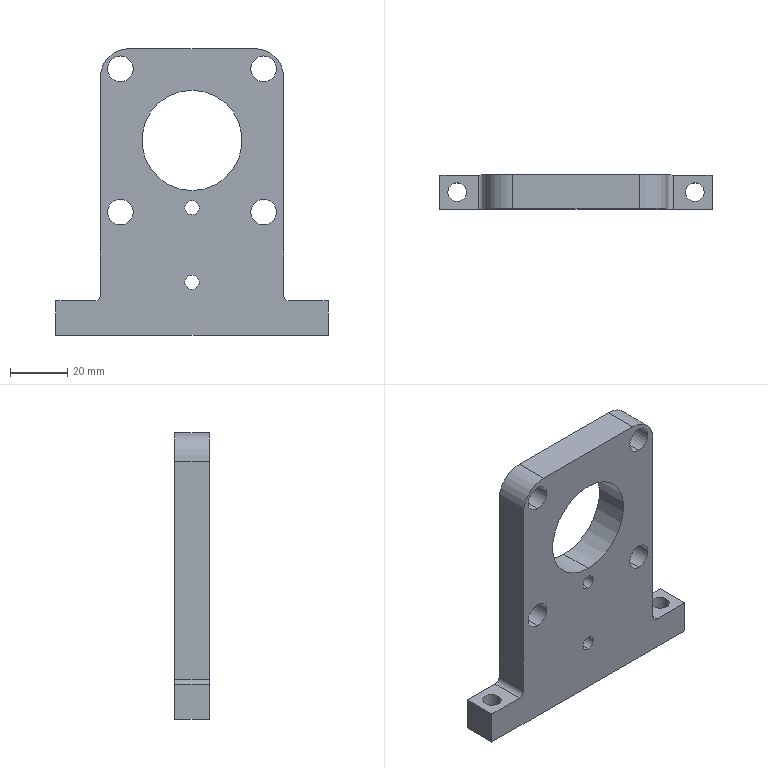Part | SolidWorks | features HoleWzd 6, ICE 3, Fillet 2, Extrusion 1 | 1 solid | 40 faces | box 95 x 12 x 100 mm | volume 64491 mm3 | cylinder 26 | plane 10 | cone 4 | commonest cylinder face diameters 5 x8 9 x8 6.5 x4 4 x2 20 x2 35 x2
STEP:
#1=CARTESIAN_POINT('',(47.5,12.,21.));
#2=VERTEX_POINT('',#1);
#3=CARTESIAN_POINT('',(47.5,12.,16.));
#4=VERTEX_POINT('',#3);
#5=CARTESIAN_POINT('',(47.5,12.,18.5));
#6=DIRECTION('',(0.,-1.,0.));
#7=DIRECTION('',(0.,0.,-1.));
#8=AXIS2_PLACEMENT_3D('',#5,#6,#7);
#9=CIRCLE('',#8,2.5);
#10=EDGE_CURVE('',#2,#4,#9,.T.);
#11=ORIENTED_EDGE('',*,*,#10,.F.);
#12=CARTESIAN_POINT('',(47.5,0.,21.));
#13=VERTEX_POINT('',#12);
#14=CARTESIAN_POINT('',(47.5,0.,21.));
#15=DIRECTION('',(0.,-1.,0.));
#16=VECTOR('',#15,1000.);
#17=LINE('',#14,#16);
#18=EDGE_CURVE('',#2,#13,#17,.T.);
#19=ORIENTED_EDGE('',*,*,#18,.T.);
#20=CARTESIAN_POINT('',(47.5,0.,16.));
#21=VERTEX_POINT('',#20);
#22=CARTESIAN_POINT('',(47.5,0.,18.5));
#23=DIRECTION('',(0.,-1.,0.));
#24=DIRECTION('',(0.,0.,-1.));
#25=AXIS2_PLACEMENT_3D('',#22,#23,#24);
#26=CIRCLE('',#25,2.5);
#27=EDGE_CURVE('',#13,#21,#26,.T.);
#28=ORIENTED_EDGE('',*,*,#27,.T.);
#29=CARTESIAN_POINT('',(47.5,0.,16.));
#30=DIRECTION('',(0.,-1.,0.));
#31=VECTOR('',#30,1000.);
#32=LINE('',#29,#31);
#33=EDGE_CURVE('',#4,#21,#32,.T.);
#34=ORIENTED_EDGE('',*,*,#33,.F.);
#35=EDGE_LOOP('',(#11,#19,#28,#34));
#36=FACE_OUTER_BOUND('',#35,.T.);
#37=CARTESIAN_POINT('',(47.5,0.,18.5));
#38=DIRECTION('',(0.,-1.,0.));
#39=DIRECTION('',(0.,0.,-1.));
#40=AXIS2_PLACEMENT_3D('',#37,#38,#39);
#41=CYLINDRICAL_SURFACE('',#40,2.5);
#42=ADVANCED_FACE('',(#36),#41,.F.);
#43=CARTESIAN_POINT('',(47.5,12.,47.));
#44=VERTEX_POINT('',#43);
#45=CARTESIAN_POINT('',(47.5,12.,42.));
#46=VERTEX_POINT('',#45);
#47=CARTESIAN_POINT('',(47.5,12.,44.5));
#48=DIRECTION('',(0.,-1.,0.));
#49=DIRECTION('',(0.,0.,-1.));
#50=AXIS2_PLACEMENT_3D('',#47,#48,#49);
#51=CIRCLE('',#50,2.5);
#52=EDGE_CURVE('',#44,#46,#51,.T.);
#53=ORIENTED_EDGE('',*,*,#52,.F.);
#54=CARTESIAN_POINT('',(47.5,0.,47.));
#55=VERTEX_POINT('',#54);
#56=CARTESIAN_POINT('',(47.5,0.,47.));
#57=DIRECTION('',(0.,-1.,0.));
#58=VECTOR('',#57,1000.);
#59=LINE('',#56,#58);
#60=EDGE_CURVE('',#44,#55,#59,.T.);
#61=ORIENTED_EDGE('',*,*,#60,.T.);
#62=CARTESIAN_POINT('',(47.5,0.,42.));
#63=VERTEX_POINT('',#62);
#64=CARTESIAN_POINT('',(47.5,0.,44.5));
#65=DIRECTION('',(0.,-1.,0.));
#66=DIRECTION('',(0.,0.,-1.));
#67=AXIS2_PLACEMENT_3D('',#64,#65,#66);
#68=CIRCLE('',#67,2.5);
#69=EDGE_CURVE('',#55,#63,#68,.T.);
#70=ORIENTED_EDGE('',*,*,#69,.T.);
#71=CARTESIAN_POINT('',(47.5,0.,42.));
#72=DIRECTION('',(0.,-1.,0.));
#73=VECTOR('',#72,1000.);
#74=LINE('',#71,#73);
#75=EDGE_CURVE('',#46,#63,#74,.T.);
#76=ORIENTED_EDGE('',*,*,#75,.F.);
#77=EDGE_LOOP('',(#53,#61,#70,#76));
#78=FACE_OUTER_BOUND('',#77,.T.);
#79=CARTESIAN_POINT('',(47.5,0.,44.5));
#80=DIRECTION('',(0.,-1.,0.));
#81=DIRECTION('',(0.,0.,-1.));
#82=AXIS2_PLACEMENT_3D('',#79,#80,#81);
#83=CYLINDRICAL_SURFACE('',#82,2.5);
#84=ADVANCED_FACE('',(#78),#83,.F.);
#85=CARTESIAN_POINT('',(72.5,12.,47.5));
#86=VERTEX_POINT('',#85);
#87=CARTESIAN_POINT('',(72.5,12.,38.5));
#88=VERTEX_POINT('',#87);
#89=CARTESIAN_POINT('',(72.5,12.,43.));
#90=DIRECTION('',(0.,-1.,0.));
#91=DIRECTION('',(0.,0.,-1.));
#92=AXIS2_PLACEMENT_3D('',#89,#90,#91);
#93=CIRCLE('',#92,4.5);
#94=EDGE_CURVE('',#86,#88,#93,.T.);
#95=ORIENTED_EDGE('',*,*,#94,.F.);
#96=CARTESIAN_POINT('',(72.5,0.,47.5));
#97=VERTEX_POINT('',#96);
#98=CARTESIAN_POINT('',(72.5,0.,47.5));
#99=DIRECTION('',(0.,-1.,0.));
#100=VECTOR('',#99,1000.);
#101=LINE('',#98,#100);
#102=EDGE_CURVE('',#86,#97,#101,.T.);
#103=ORIENTED_EDGE('',*,*,#102,.T.);
#104=CARTESIAN_POINT('',(72.5,0.,38.5));
#105=VERTEX_POINT('',#104);
#106=CARTESIAN_POINT('',(72.5,0.,43.));
#107=DIRECTION('',(0.,-1.,0.));
#108=DIRECTION('',(0.,0.,-1.));
#109=AXIS2_PLACEMENT_3D('',#106,#107,#108);
#110=CIRCLE('',#109,4.5);
#111=EDGE_CURVE('',#97,#105,#110,.T.);
#112=ORIENTED_EDGE('',*,*,#111,.T.);
#113=CARTESIAN_POINT('',(72.5,0.,38.5));
#114=DIRECTION('',(0.,-1.,0.));
#115=VECTOR('',#114,1000.);
#116=LINE('',#113,#115);
#117=EDGE_CURVE('',#88,#105,#116,.T.);
#118=ORIENTED_EDGE('',*,*,#117,.F.);
#119=EDGE_LOOP('',(#95,#103,#112,#118));
#120=FACE_OUTER_BOUND('',#119,.T.);
#121=CARTESIAN_POINT('',(72.5,0.,43.));
#122=DIRECTION('',(0.,-1.,0.));
#123=DIRECTION('',(0.,0.,-1.));
#124=AXIS2_PLACEMENT_3D('',#121,#122,#123);
#125=CYLINDRICAL_SURFACE('',#124,4.5);
#126=ADVANCED_FACE('',(#120),#125,.F.);
#127=CARTESIAN_POINT('',(72.5,12.,97.5));
#128=VERTEX_POINT('',#127);
#129=CARTESIAN_POINT('',(72.5,12.,88.5));
#130=VERTEX_POINT('',#129);
#131=CARTESIAN_POINT('',(72.5,12.,93.));
#132=DIRECTION('',(0.,-1.,0.));
#133=DIRECTION('',(0.,0.,-1.));
#134=AXIS2_PLACEMENT_3D('',#131,#132,#133);
#135=CIRCLE('',#134,4.5);
#136=EDGE_CURVE('',#128,#130,#135,.T.);
#137=ORIENTED_EDGE('',*,*,#136,.F.);
#138=CARTESIAN_POINT('',(72.5,0.,97.5));
#139=VERTEX_POINT('',#138);
#140=CARTESIAN_POINT('',(72.5,0.,97.5));
#141=DIRECTION('',(0.,-1.,0.));
#142=VECTOR('',#141,1000.);
#143=LINE('',#140,#142);
#144=EDGE_CURVE('',#128,#139,#143,.T.);
#145=ORIENTED_EDGE('',*,*,#144,.T.);
#146=CARTESIAN_POINT('',(72.5,0.,88.5));
#147=VERTEX_POINT('',#146);
#148=CARTESIAN_POINT('',(72.5,0.,93.));
#149=DIRECTION('',(0.,-1.,0.));
#150=DIRECTION('',(0.,0.,-1.));
#151=AXIS2_PLACEMENT_3D('',#148,#149,#150);
#152=CIRCLE('',#151,4.5);
#153=EDGE_CURVE('',#139,#147,#152,.T.);
#154=ORIENTED_EDGE('',*,*,#153,.T.);
#155=CARTESIAN_POINT('',(72.5,0.,88.5));
#156=DIRECTION('',(0.,-1.,0.));
#157=VECTOR('',#156,1000.);
#158=LINE('',#155,#157);
#159=EDGE_CURVE('',#130,#147,#158,.T.);
#160=ORIENTED_EDGE('',*,*,#159,.F.);
#161=EDGE_LOOP('',(#137,#145,#154,#160));
#162=FACE_OUTER_BOUND('',#161,.T.);
#163=CARTESIAN_POINT('',(72.5,0.,93.));
#164=DIRECTION('',(0.,-1.,0.));
#165=DIRECTION('',(0.,0.,-1.));
#166=AXIS2_PLACEMENT_3D('',#163,#164,#165);
#167=CYLINDRICAL_SURFACE('',#166,4.5);
#168=ADVANCED_FACE('',(#162),#167,.F.);
#169=CARTESIAN_POINT('',(22.5,12.,97.5));
#170=VERTEX_POINT('',#169);
#171=CARTESIAN_POINT('',(22.5,12.,88.5));
#172=VERTEX_POINT('',#171);
#173=CARTESIAN_POINT('',(22.5,12.,93.));
#174=DIRECTION('',(0.,-1.,0.));
#175=DIRECTION('',(0.,0.,-1.));
#176=AXIS2_PLACEMENT_3D('',#173,#174,#175);
#177=CIRCLE('',#176,4.5);
#178=EDGE_CURVE('',#170,#172,#177,.T.);
#179=ORIENTED_EDGE('',*,*,#178,.F.);
#180=CARTESIAN_POINT('',(22.5,0.,97.5));
#181=VERTEX_POINT('',#180);
#182=CARTESIAN_POINT('',(22.5,0.,97.5));
#183=DIRECTION('',(0.,-1.,0.));
#184=VECTOR('',#183,1000.);
#185=LINE('',#182,#184);
#186=EDGE_CURVE('',#170,#181,#185,.T.);
#187=ORIENTED_EDGE('',*,*,#186,.T.);
#188=CARTESIAN_POINT('',(22.5,0.,88.5));
#189=VERTEX_POINT('',#188);
#190=CARTESIAN_POINT('',(22.5,0.,93.));
#191=DIRECTION('',(0.,-1.,0.));
#192=DIRECTION('',(0.,0.,-1.));
#193=AXIS2_PLACEMENT_3D('',#190,#191,#192);
#194=CIRCLE('',#193,4.5);
#195=EDGE_CURVE('',#181,#189,#194,.T.);
#196=ORIENTED_EDGE('',*,*,#195,.T.);
#197=CARTESIAN_POINT('',(22.5,0.,88.5));
#198=DIRECTION('',(0.,-1.,0.));
#199=VECTOR('',#198,1000.);
#200=LINE('',#197,#199);
#201=EDGE_CURVE('',#172,#189,#200,.T.);
#202=ORIENTED_EDGE('',*,*,#201,.F.);
#203=EDGE_LOOP('',(#179,#187,#196,#202));
#204=FACE_OUTER_BOUND('',#203,.T.);
#205=CARTESIAN_POINT('',(22.5,0.,93.));
#206=DIRECTION('',(0.,-1.,0.));
#207=DIRECTION('',(0.,0.,-1.));
#208=AXIS2_PLACEMENT_3D('',#205,#206,#207);
#209=CYLINDRICAL_SURFACE('',#208,4.5);
#210=ADVANCED_FACE('',(#204),#209,.F.);
#211=CARTESIAN_POINT('',(22.5,12.,47.5));
#212=VERTEX_POINT('',#211);
#213=CARTESIAN_POINT('',(22.5,12.,38.5));
#214=VERTEX_POINT('',#213);
#215=CARTESIAN_POINT('',(22.5,12.,43.));
#216=DIRECTION('',(0.,-1.,0.));
#217=DIRECTION('',(0.,0.,-1.));
#218=AXIS2_PLACEMENT_3D('',#215,#216,#217);
#219=CIRCLE('',#218,4.5);
#220=EDGE_CURVE('',#212,#214,#219,.T.);
#221=ORIENTED_EDGE('',*,*,#220,.F.);
#222=CARTESIAN_POINT('',(22.5,0.,47.5));
#223=VERTEX_POINT('',#222);
#224=CARTESIAN_POINT('',(22.5,0.,47.5));
#225=DIRECTION('',(0.,-1.,0.));
#226=VECTOR('',#225,1000.);
#227=LINE('',#224,#226);
#228=EDGE_CURVE('',#212,#223,#227,.T.);
#229=ORIENTED_EDGE('',*,*,#228,.T.);
#230=CARTESIAN_POINT('',(22.5,0.,38.5));
#231=VERTEX_POINT('',#230);
#232=CARTESIAN_POINT('',(22.5,0.,43.));
#233=DIRECTION('',(0.,-1.,0.));
#234=DIRECTION('',(0.,0.,-1.));
#235=AXIS2_PLACEMENT_3D('',#232,#233,#234);
#236=CIRCLE('',#235,4.5);
#237=EDGE_CURVE('',#223,#231,#236,.T.);
#238=ORIENTED_EDGE('',*,*,#237,.T.);
#239=CARTESIAN_POINT('',(22.5,0.,38.5));
#240=DIRECTION('',(0.,-1.,0.));
#241=VECTOR('',#240,1000.);
#242=LINE('',#239,#241);
#243=EDGE_CURVE('',#214,#231,#242,.T.);
#244=ORIENTED_EDGE('',*,*,#243,.F.);
#245=EDGE_LOOP('',(#221,#229,#238,#244));
#246=FACE_OUTER_BOUND('',#245,.T.);
#247=CARTESIAN_POINT('',(22.5,0.,43.));
#248=DIRECTION('',(0.,-1.,0.));
#249=DIRECTION('',(0.,0.,-1.));
#250=AXIS2_PLACEMENT_3D('',#247,#248,#249);
#251=CYLINDRICAL_SURFACE('',#250,4.5);
#252=ADVANCED_FACE('',(#246),#251,.F.);
#253=CARTESIAN_POINT('',(70.,6.,10.));
#254=VERTEX_POINT('',#253);
#255=CARTESIAN_POINT('',(65.,6.,10.));
#256=VERTEX_POINT('',#255);
#257=CARTESIAN_POINT('',(67.5,6.,10.));
#258=DIRECTION('',(0.,0.,-1.));
#259=DIRECTION('',(-1.,0.,0.));
#260=AXIS2_PLACEMENT_3D('',#257,#258,#259);
#261=CIRCLE('',#260,2.5);
#262=EDGE_CURVE('',#254,#256,#261,.T.);
#263=ORIENTED_EDGE('',*,*,#262,.F.);
#264=CARTESIAN_POINT('',(70.,6.,0.));
#265=VERTEX_POINT('',#264);
#266=CARTESIAN_POINT('',(70.,6.,0.));
#267=DIRECTION('',(0.,0.,-1.));
#268=VECTOR('',#267,1000.);
#269=LINE('',#266,#268);
#270=EDGE_CURVE('',#254,#265,#269,.T.);
#271=ORIENTED_EDGE('',*,*,#270,.T.);
#272=CARTESIAN_POINT('',(65.,6.,0.));
#273=VERTEX_POINT('',#272);
#274=CARTESIAN_POINT('',(67.5,6.,0.));
#275=DIRECTION('',(0.,0.,-1.));
#276=DIRECTION('',(-1.,0.,0.));
#277=AXIS2_PLACEMENT_3D('',#274,#275,#276);
#278=CIRCLE('',#277,2.5);
#279=EDGE_CURVE('',#265,#273,#278,.T.);
#280=ORIENTED_EDGE('',*,*,#279,.T.);
#281=CARTESIAN_POINT('',(65.,6.,0.));
#282=DIRECTION('',(0.,0.,-1.));
#283=VECTOR('',#282,1000.);
#284=LINE('',#281,#283);
#285=EDGE_CURVE('',#256,#273,#284,.T.);
#286=ORIENTED_EDGE('',*,*,#285,.F.);
#287=EDGE_LOOP('',(#263,#271,#280,#286));
#288=FACE_OUTER_BOUND('',#287,.T.);
#289=CARTESIAN_POINT('',(67.5,6.,0.));
#290=DIRECTION('',(0.,0.,-1.));
#291=DIRECTION('',(-1.,0.,0.));
#292=AXIS2_PLACEMENT_3D('',#289,#290,#291);
#293=CYLINDRICAL_SURFACE('',#292,2.5);
#294=ADVANCED_FACE('',(#288),#293,.F.);
#295=CARTESIAN_POINT('',(67.5,6.,11.502));
#296=VERTEX_POINT('',#295);
#297=CARTESIAN_POINT('',(65.,6.,10.));
#298=DIRECTION('',(-0.8572,0.,-0.515));
#299=VECTOR('',#298,1000.);
#300=LINE('',#297,#299);
#301=EDGE_CURVE('',#296,#256,#300,.T.);
#302=ORIENTED_EDGE('',*,*,#301,.F.);
#303=CARTESIAN_POINT('',(70.,6.,10.));
#304=DIRECTION('',(0.8572,0.,-0.515));
#305=VECTOR('',#304,1000.);
#306=LINE('',#303,#305);
#307=EDGE_CURVE('',#296,#254,#306,.T.);
#308=ORIENTED_EDGE('',*,*,#307,.T.);
#309=ORIENTED_EDGE('',*,*,#262,.T.);
#310=EDGE_LOOP('',(#302,#308,#309));
#311=FACE_OUTER_BOUND('',#310,.T.);
#312=CARTESIAN_POINT('',(67.5,6.,10.));
#313=DIRECTION('',(0.,0.,-1.));
#314=DIRECTION('',(-1.,0.,0.));
#315=AXIS2_PLACEMENT_3D('',#312,#313,#314);
#316=CONICAL_SURFACE('',#315,2.5,1.03);
#317=ADVANCED_FACE('',(#311),#316,.F.);
#318=CARTESIAN_POINT('',(30.,6.,10.));
#319=VERTEX_POINT('',#318);
#320=CARTESIAN_POINT('',(25.,6.,10.));
#321=VERTEX_POINT('',#320);
#322=CARTESIAN_POINT('',(27.5,6.,10.));
#323=DIRECTION('',(0.,0.,-1.));
#324=DIRECTION('',(-1.,0.,0.));
#325=AXIS2_PLACEMENT_3D('',#322,#323,#324);
#326=CIRCLE('',#325,2.5);
#327=EDGE_CURVE('',#319,#321,#326,.T.);
#328=ORIENTED_EDGE('',*,*,#327,.F.);
#329=CARTESIAN_POINT('',(30.,6.,0.));
#330=VERTEX_POINT('',#329);
#331=CARTESIAN_POINT('',(30.,6.,0.));
#332=DIRECTION('',(0.,0.,-1.));
#333=VECTOR('',#332,1000.);
#334=LINE('',#331,#333);
#335=EDGE_CURVE('',#319,#330,#334,.T.);
#336=ORIENTED_EDGE('',*,*,#335,.T.);
#337=CARTESIAN_POINT('',(25.,6.,0.));
#338=VERTEX_POINT('',#337);
#339=CARTESIAN_POINT('',(27.5,6.,0.));
#340=DIRECTION('',(0.,0.,-1.));
#341=DIRECTION('',(-1.,0.,0.));
#342=AXIS2_PLACEMENT_3D('',#339,#340,#341);
#343=CIRCLE('',#342,2.5);
#344=EDGE_CURVE('',#330,#338,#343,.T.);
#345=ORIENTED_EDGE('',*,*,#344,.T.);
#346=CARTESIAN_POINT('',(25.,6.,0.));
#347=DIRECTION('',(0.,0.,-1.));
#348=VECTOR('',#347,1000.);
#349=LINE('',#346,#348);
#350=EDGE_CURVE('',#321,#338,#349,.T.);
#351=ORIENTED_EDGE('',*,*,#350,.F.);
#352=EDGE_LOOP('',(#328,#336,#345,#351));
#353=FACE_OUTER_BOUND('',#352,.T.);
#354=CARTESIAN_POINT('',(27.5,6.,0.));
#355=DIRECTION('',(0.,0.,-1.));
#356=DIRECTION('',(-1.,0.,0.));
#357=AXIS2_PLACEMENT_3D('',#354,#355,#356);
#358=CYLINDRICAL_SURFACE('',#357,2.5);
#359=ADVANCED_FACE('',(#353),#358,.F.);
#360=CARTESIAN_POINT('',(27.5,6.,11.502));
#361=VERTEX_POINT('',#360);
#362=CARTESIAN_POINT('',(25.,6.,10.));
#363=DIRECTION('',(-0.8572,0.,-0.515));
#364=VECTOR('',#363,1000.);
#365=LINE('',#362,#364);
#366=EDGE_CURVE('',#361,#321,#365,.T.);
#367=ORIENTED_EDGE('',*,*,#366,.F.);
#368=CARTESIAN_POINT('',(30.,6.,10.));
#369=DIRECTION('',(0.8572,0.,-0.515));
#370=VECTOR('',#369,1000.);
#371=LINE('',#368,#370);
#372=EDGE_CURVE('',#361,#319,#371,.T.);
#373=ORIENTED_EDGE('',*,*,#372,.T.);
#374=ORIENTED_EDGE('',*,*,#327,.T.);
#375=EDGE_LOOP('',(#367,#373,#374));
#376=FACE_OUTER_BOUND('',#375,.T.);
#377=CARTESIAN_POINT('',(27.5,6.,10.));
#378=DIRECTION('',(0.,0.,-1.));
#379=DIRECTION('',(-1.,0.,0.));
#380=AXIS2_PLACEMENT_3D('',#377,#378,#379);
#381=CONICAL_SURFACE('',#380,2.5,1.03);
#382=ADVANCED_FACE('',(#376),#381,.F.);
#383=CARTESIAN_POINT('',(47.5,0.,50.5));
#384=VERTEX_POINT('',#383);
#385=CARTESIAN_POINT('',(47.5,0.,85.5));
#386=VERTEX_POINT('',#385);
#387=CARTESIAN_POINT('',(47.5,0.,68.));
#388=DIRECTION('',(0.,1.,0.));
#389=DIRECTION('',(0.,0.,1.));
#390=AXIS2_PLACEMENT_3D('',#387,#388,#389);
#391=CIRCLE('',#390,17.5);
#392=EDGE_CURVE('',#384,#386,#391,.T.);
#393=ORIENTED_EDGE('',*,*,#392,.F.);
#394=CARTESIAN_POINT('',(47.5,12.,50.5));
#395=VERTEX_POINT('',#394);
#396=CARTESIAN_POINT('',(47.5,0.,50.5));
#397=DIRECTION('',(0.,1.,0.));
#398=VECTOR('',#397,1000.);
#399=LINE('',#396,#398);
#400=EDGE_CURVE('',#384,#395,#399,.T.);
#401=ORIENTED_EDGE('',*,*,#400,.T.);
#402=CARTESIAN_POINT('',(47.5,12.,85.5));
#403=VERTEX_POINT('',#402);
#404=CARTESIAN_POINT('',(47.5,12.,68.));
#405=DIRECTION('',(0.,1.,0.));
#406=DIRECTION('',(0.,0.,1.));
#407=AXIS2_PLACEMENT_3D('',#404,#405,#406);
#408=CIRCLE('',#407,17.5);
#409=EDGE_CURVE('',#395,#403,#408,.T.);
#410=ORIENTED_EDGE('',*,*,#409,.T.);
#411=CARTESIAN_POINT('',(47.5,0.,85.5));
#412=DIRECTION('',(0.,1.,0.));
#413=VECTOR('',#412,1000.);
#414=LINE('',#411,#413);
#415=EDGE_CURVE('',#386,#403,#414,.T.);
#416=ORIENTED_EDGE('',*,*,#415,.F.);
#417=EDGE_LOOP('',(#393,#401,#410,#416));
#418=FACE_OUTER_BOUND('',#417,.T.);
#419=CARTESIAN_POINT('',(47.5,0.,68.));
#420=DIRECTION('',(0.,1.,0.));
#421=DIRECTION('',(0.,0.,1.));
#422=AXIS2_PLACEMENT_3D('',#419,#420,#421);
#423=CYLINDRICAL_SURFACE('',#422,17.5);
#424=ADVANCED_FACE('',(#418),#423,.F.);
#425=CARTESIAN_POINT('',(2.75,6.,0.));
#426=VERTEX_POINT('',#425);
#427=CARTESIAN_POINT('',(9.25,6.,0.));
#428=VERTEX_POINT('',#427);
#429=CARTESIAN_POINT('',(6.,6.,0.));
#430=DIRECTION('',(0.,0.,1.));
#431=DIRECTION('',(1.,0.,0.));
#432=AXIS2_PLACEMENT_3D('',#429,#430,#431);
#433=CIRCLE('',#432,3.25);
#434=EDGE_CURVE('',#426,#428,#433,.T.);
#435=ORIENTED_EDGE('',*,*,#434,.F.);
#436=CARTESIAN_POINT('',(2.75,6.,12.));
#437=VERTEX_POINT('',#436);
#438=CARTESIAN_POINT('',(2.75,6.,12.));
#439=DIRECTION('',(0.,0.,1.));
#440=VECTOR('',#439,1000.);
#441=LINE('',#438,#440);
#442=EDGE_CURVE('',#426,#437,#441,.T.);
#443=ORIENTED_EDGE('',*,*,#442,.T.);
#444=CARTESIAN_POINT('',(9.25,6.,12.));
#445=VERTEX_POINT('',#444);
#446=CARTESIAN_POINT('',(6.,6.,12.));
#447=DIRECTION('',(0.,0.,1.));
#448=DIRECTION('',(1.,0.,0.));
#449=AXIS2_PLACEMENT_3D('',#446,#447,#448);
#450=CIRCLE('',#449,3.25);
#451=EDGE_CURVE('',#437,#445,#450,.T.);
#452=ORIENTED_EDGE('',*,*,#451,.T.);
#453=CARTESIAN_POINT('',(9.25,6.,12.));
#454=DIRECTION('',(0.,0.,1.));
#455=VECTOR('',#454,1000.);
#456=LINE('',#453,#455);
#457=EDGE_CURVE('',#428,#445,#456,.T.);
#458=ORIENTED_EDGE('',*,*,#457,.F.);
#459=EDGE_LOOP('',(#435,#443,#452,#458));
#460=FACE_OUTER_BOUND('',#459,.T.);
#461=CARTESIAN_POINT('',(6.,6.,12.));
#462=DIRECTION('',(0.,0.,1.));
#463=DIRECTION('',(1.,0.,0.));
#464=AXIS2_PLACEMENT_3D('',#461,#462,#463);
#465=CYLINDRICAL_SURFACE('',#464,3.25);
#466=ADVANCED_FACE('',(#460),#465,.F.);
#467=CARTESIAN_POINT('',(85.75,6.,0.));
#468=VERTEX_POINT('',#467);
#469=CARTESIAN_POINT('',(92.25,6.,0.));
#470=VERTEX_POINT('',#469);
#471=CARTESIAN_POINT('',(89.,6.,0.));
#472=DIRECTION('',(0.,0.,1.));
#473=DIRECTION('',(1.,0.,0.));
#474=AXIS2_PLACEMENT_3D('',#471,#472,#473);
#475=CIRCLE('',#474,3.25);
#476=EDGE_CURVE('',#468,#470,#475,.T.);
#477=ORIENTED_EDGE('',*,*,#476,.F.);
#478=CARTESIAN_POINT('',(85.75,6.,12.));
#479=VERTEX_POINT('',#478);
#480=CARTESIAN_POINT('',(85.75,6.,12.));
#481=DIRECTION('',(0.,0.,1.));
#482=VECTOR('',#481,1000.);
#483=LINE('',#480,#482);
#484=EDGE_CURVE('',#468,#479,#483,.T.);
#485=ORIENTED_EDGE('',*,*,#484,.T.);
#486=CARTESIAN_POINT('',(92.25,6.,12.));
#487=VERTEX_POINT('',#486);
#488=CARTESIAN_POINT('',(89.,6.,12.));
#489=DIRECTION('',(0.,0.,1.));
#490=DIRECTION('',(1.,0.,0.));
#491=AXIS2_PLACEMENT_3D('',#488,#489,#490);
#492=CIRCLE('',#491,3.25);
#493=EDGE_CURVE('',#479,#487,#492,.T.);
#494=ORIENTED_EDGE('',*,*,#493,.T.);
#495=CARTESIAN_POINT('',(92.25,6.,12.));
#496=DIRECTION('',(0.,0.,1.));
#497=VECTOR('',#496,1000.);
#498=LINE('',#495,#497);
#499=EDGE_CURVE('',#470,#487,#498,.T.);
#500=ORIENTED_EDGE('',*,*,#499,.F.);
#501=EDGE_LOOP('',(#477,#485,#494,#500));
#502=FACE_OUTER_BOUND('',#501,.T.);
#503=CARTESIAN_POINT('',(89.,6.,12.));
#504=DIRECTION('',(0.,0.,1.));
#505=DIRECTION('',(1.,0.,0.));
#506=AXIS2_PLACEMENT_3D('',#503,#504,#505);
#507=CYLINDRICAL_SURFACE('',#506,3.25);
#508=ADVANCED_FACE('',(#502),#507,.F.);
#509=CARTESIAN_POINT('',(0.,0.,0.));
#510=VERTEX_POINT('',#509);
#511=CARTESIAN_POINT('',(0.,0.,12.));
#512=VERTEX_POINT('',#511);
#513=CARTESIAN_POINT('',(0.,0.,100.));
#514=DIRECTION('',(0.,0.,1.));
#515=VECTOR('',#514,1000.);
#516=LINE('',#513,#515);
#517=EDGE_CURVE('',#510,#512,#516,.T.);
#518=ORIENTED_EDGE('',*,*,#517,.T.);
#519=CARTESIAN_POINT('',(0.,12.,12.));
#520=VERTEX_POINT('',#519);
#521=CARTESIAN_POINT('',(0.,0.,12.));
#522=DIRECTION('',(0.,1.,0.));
#523=VECTOR('',#522,1000.);
#524=LINE('',#521,#523);
#525=EDGE_CURVE('',#512,#520,#524,.T.);
#526=ORIENTED_EDGE('',*,*,#525,.T.);
#527=CARTESIAN_POINT('',(0.,12.,0.));
#528=VERTEX_POINT('',#527);
#529=CARTESIAN_POINT('',(0.,12.,100.));
#530=DIRECTION('',(0.,0.,1.));
#531=VECTOR('',#530,1000.);
#532=LINE('',#529,#531);
#533=EDGE_CURVE('',#528,#520,#532,.T.);
#534=ORIENTED_EDGE('',*,*,#533,.F.);
#535=CARTESIAN_POINT('',(0.,12.,0.));
#536=DIRECTION('',(0.,-1.,0.));
#537=VECTOR('',#536,1000.);
#538=LINE('',#535,#537);
#539=EDGE_CURVE('',#528,#510,#538,.T.);
#540=ORIENTED_EDGE('',*,*,#539,.T.);
#541=EDGE_LOOP('',(#518,#526,#534,#540));
#542=FACE_OUTER_BOUND('',#541,.T.);
#543=CARTESIAN_POINT('',(0.,12.,100.));
#544=DIRECTION('',(1.,0.,0.));
#545=DIRECTION('',(0.,0.,-1.));
#546=AXIS2_PLACEMENT_3D('',#543,#544,#545);
#547=PLANE('',#546);
#548=ADVANCED_FACE('',(#542),#547,.F.);
#549=CARTESIAN_POINT('',(25.5,12.,100.));
#550=VERTEX_POINT('',#549);
#551=CARTESIAN_POINT('',(69.5,12.,100.));
#552=VERTEX_POINT('',#551);
#553=CARTESIAN_POINT('',(95.,12.,100.));
#554=DIRECTION('',(1.,0.,0.));
#555=VECTOR('',#554,1000.);
#556=LINE('',#553,#555);
#557=EDGE_CURVE('',#550,#552,#556,.T.);
#558=ORIENTED_EDGE('',*,*,#557,.F.);
#559=CARTESIAN_POINT('',(25.5,0.,100.));
#560=VERTEX_POINT('',#559);
#561=CARTESIAN_POINT('',(25.5,12.,100.));
#562=DIRECTION('',(0.,-1.,0.));
#563=VECTOR('',#562,1000.);
#564=LINE('',#561,#563);
#565=EDGE_CURVE('',#550,#560,#564,.T.);
#566=ORIENTED_EDGE('',*,*,#565,.T.);
#567=CARTESIAN_POINT('',(69.5,0.,100.));
#568=VERTEX_POINT('',#567);
#569=CARTESIAN_POINT('',(95.,0.,100.));
#570=DIRECTION('',(1.,0.,0.));
#571=VECTOR('',#570,1000.);
#572=LINE('',#569,#571);
#573=EDGE_CURVE('',#560,#568,#572,.T.);
#574=ORIENTED_EDGE('',*,*,#573,.T.);
#575=CARTESIAN_POINT('',(69.5,12.,100.));
#576=DIRECTION('',(0.,1.,0.));
#577=VECTOR('',#576,1000.);
#578=LINE('',#575,#577);
#579=EDGE_CURVE('',#568,#552,#578,.T.);
#580=ORIENTED_EDGE('',*,*,#579,.T.);
#581=EDGE_LOOP('',(#558,#566,#574,#580));
#582=FACE_OUTER_BOUND('',#581,.T.);
#583=CARTESIAN_POINT('',(95.,12.,100.));
#584=DIRECTION('',(0.,0.,-1.));
#585=DIRECTION('',(-1.,0.,0.));
#586=AXIS2_PLACEMENT_3D('',#583,#584,#585);
#587=PLANE('',#586);
#588=ADVANCED_FACE('',(#582),#587,.F.);
#589=CARTESIAN_POINT('',(95.,12.,12.));
#590=VERTEX_POINT('',#589);
#591=CARTESIAN_POINT('',(95.,12.,0.));
#592=VERTEX_POINT('',#591);
#593=CARTESIAN_POINT('',(95.,12.,0.));
#594=DIRECTION('',(0.,0.,-1.));
#595=VECTOR('',#594,1000.);
#596=LINE('',#593,#595);
#597=EDGE_CURVE('',#590,#592,#596,.T.);
#598=ORIENTED_EDGE('',*,*,#597,.F.);
#599=CARTESIAN_POINT('',(95.,0.,12.));
#600=VERTEX_POINT('',#599);
#601=CARTESIAN_POINT('',(95.,0.,12.));
#602=DIRECTION('',(0.,1.,0.));
#603=VECTOR('',#602,1000.);
#604=LINE('',#601,#603);
#605=EDGE_CURVE('',#600,#590,#604,.T.);
#606=ORIENTED_EDGE('',*,*,#605,.F.);
#607=CARTESIAN_POINT('',(95.,0.,0.));
#608=VERTEX_POINT('',#607);
#609=CARTESIAN_POINT('',(95.,0.,0.));
#610=DIRECTION('',(0.,0.,-1.));
#611=VECTOR('',#610,1000.);
#612=LINE('',#609,#611);
#613=EDGE_CURVE('',#600,#608,#612,.T.);
#614=ORIENTED_EDGE('',*,*,#613,.T.);
#615=CARTESIAN_POINT('',(95.,12.,0.));
#616=DIRECTION('',(0.,-1.,0.));
#617=VECTOR('',#616,1000.);
#618=LINE('',#615,#617);
#619=EDGE_CURVE('',#592,#608,#618,.T.);
#620=ORIENTED_EDGE('',*,*,#619,.F.);
#621=EDGE_LOOP('',(#598,#606,#614,#620));
#622=FACE_OUTER_BOUND('',#621,.T.);
#623=CARTESIAN_POINT('',(95.,12.,0.));
#624=DIRECTION('',(-1.,0.,0.));
#625=DIRECTION('',(0.,0.,1.));
#626=AXIS2_PLACEMENT_3D('',#623,#624,#625);
#627=PLANE('',#626);
#628=ADVANCED_FACE('',(#622),#627,.F.);
#629=CARTESIAN_POINT('',(67.5,6.,0.));
#630=DIRECTION('',(0.,0.,-1.));
#631=DIRECTION('',(-1.,0.,0.));
#632=AXIS2_PLACEMENT_3D('',#629,#630,#631);
#633=CIRCLE('',#632,2.5);
#634=EDGE_CURVE('',#273,#265,#633,.T.);
#635=ORIENTED_EDGE('',*,*,#634,.F.);
#636=ORIENTED_EDGE('',*,*,#279,.F.);
#637=EDGE_LOOP('',(#635,#636));
#638=FACE_BOUND('',#637,.T.);
#639=CARTESIAN_POINT('',(27.5,6.,0.));
#640=DIRECTION('',(0.,0.,-1.));
#641=DIRECTION('',(-1.,0.,0.));
#642=AXIS2_PLACEMENT_3D('',#639,#640,#641);
#643=CIRCLE('',#642,2.5);
#644=EDGE_CURVE('',#338,#330,#643,.T.);
#645=ORIENTED_EDGE('',*,*,#644,.F.);
#646=ORIENTED_EDGE('',*,*,#344,.F.);
#647=EDGE_LOOP('',(#645,#646));
#648=FACE_BOUND('',#647,.T.);
#649=CARTESIAN_POINT('',(6.,6.,0.));
#650=DIRECTION('',(0.,0.,1.));
#651=DIRECTION('',(1.,0.,0.));
#652=AXIS2_PLACEMENT_3D('',#649,#650,#651);
#653=CIRCLE('',#652,3.25);
#654=EDGE_CURVE('',#428,#426,#653,.T.);
#655=ORIENTED_EDGE('',*,*,#654,.T.);
#656=ORIENTED_EDGE('',*,*,#434,.T.);
#657=EDGE_LOOP('',(#655,#656));
#658=FACE_BOUND('',#657,.T.);
#659=CARTESIAN_POINT('',(89.,6.,0.));
#660=DIRECTION('',(0.,0.,1.));
#661=DIRECTION('',(1.,0.,0.));
#662=AXIS2_PLACEMENT_3D('',#659,#660,#661);
#663=CIRCLE('',#662,3.25);
#664=EDGE_CURVE('',#470,#468,#663,.T.);
#665=ORIENTED_EDGE('',*,*,#664,.T.);
#666=ORIENTED_EDGE('',*,*,#476,.T.);
#667=EDGE_LOOP('',(#665,#666));
#668=FACE_BOUND('',#667,.T.);
#669=CARTESIAN_POINT('',(0.,0.,0.));
#670=DIRECTION('',(-1.,0.,0.));
#671=VECTOR('',#670,1000.);
#672=LINE('',#669,#671);
#673=EDGE_CURVE('',#608,#510,#672,.T.);
#674=ORIENTED_EDGE('',*,*,#673,.T.);
#675=ORIENTED_EDGE('',*,*,#539,.F.);
#676=CARTESIAN_POINT('',(0.,12.,0.));
#677=DIRECTION('',(-1.,0.,0.));
#678=VECTOR('',#677,1000.);
#679=LINE('',#676,#678);
#680=EDGE_CURVE('',#592,#528,#679,.T.);
#681=ORIENTED_EDGE('',*,*,#680,.F.);
#682=ORIENTED_EDGE('',*,*,#619,.T.);
#683=EDGE_LOOP('',(#674,#675,#681,#682));
#684=FACE_OUTER_BOUND('',#683,.T.);
#685=CARTESIAN_POINT('',(0.,12.,0.));
#686=DIRECTION('',(0.,0.,1.));
#687=DIRECTION('',(1.,0.,0.));
#688=AXIS2_PLACEMENT_3D('',#685,#686,#687);
#689=PLANE('',#688);
#690=ADVANCED_FACE('',(#638,#648,#658,#668,#684),#689,.F.);
#691=CARTESIAN_POINT('',(47.5,12.,18.5));
#692=DIRECTION('',(0.,-1.,0.));
#693=DIRECTION('',(0.,0.,-1.));
#694=AXIS2_PLACEMENT_3D('',#691,#692,#693);
#695=CIRCLE('',#694,2.5);
#696=EDGE_CURVE('',#4,#2,#695,.T.);
#697=ORIENTED_EDGE('',*,*,#696,.T.);
#698=ORIENTED_EDGE('',*,*,#10,.T.);
#699=EDGE_LOOP('',(#697,#698));
#700=FACE_BOUND('',#699,.T.);
#701=CARTESIAN_POINT('',(47.5,12.,44.5));
#702=DIRECTION('',(0.,-1.,0.));
#703=DIRECTION('',(0.,0.,-1.));
#704=AXIS2_PLACEMENT_3D('',#701,#702,#703);
#705=CIRCLE('',#704,2.5);
#706=EDGE_CURVE('',#46,#44,#705,.T.);
#707=ORIENTED_EDGE('',*,*,#706,.T.);
#708=ORIENTED_EDGE('',*,*,#52,.T.);
#709=EDGE_LOOP('',(#707,#708));
#710=FACE_BOUND('',#709,.T.);
#711=CARTESIAN_POINT('',(72.5,12.,43.));
#712=DIRECTION('',(0.,-1.,0.));
#713=DIRECTION('',(0.,0.,-1.));
#714=AXIS2_PLACEMENT_3D('',#711,#712,#713);
#715=CIRCLE('',#714,4.5);
#716=EDGE_CURVE('',#88,#86,#715,.T.);
#717=ORIENTED_EDGE('',*,*,#716,.T.);
#718=ORIENTED_EDGE('',*,*,#94,.T.);
#719=EDGE_LOOP('',(#717,#718));
#720=FACE_BOUND('',#719,.T.);
#721=CARTESIAN_POINT('',(72.5,12.,93.));
#722=DIRECTION('',(0.,-1.,0.));
#723=DIRECTION('',(0.,0.,-1.));
#724=AXIS2_PLACEMENT_3D('',#721,#722,#723);
#725=CIRCLE('',#724,4.5);
#726=EDGE_CURVE('',#130,#128,#725,.T.);
#727=ORIENTED_EDGE('',*,*,#726,.T.);
#728=ORIENTED_EDGE('',*,*,#136,.T.);
#729=EDGE_LOOP('',(#727,#728));
#730=FACE_BOUND('',#729,.T.);
#731=CARTESIAN_POINT('',(22.5,12.,93.));
#732=DIRECTION('',(0.,-1.,0.));
#733=DIRECTION('',(0.,0.,-1.));
#734=AXIS2_PLACEMENT_3D('',#731,#732,#733);
#735=CIRCLE('',#734,4.5);
#736=EDGE_CURVE('',#172,#170,#735,.T.);
#737=ORIENTED_EDGE('',*,*,#736,.T.);
#738=ORIENTED_EDGE('',*,*,#178,.T.);
#739=EDGE_LOOP('',(#737,#738));
#740=FACE_BOUND('',#739,.T.);
#741=CARTESIAN_POINT('',(22.5,12.,43.));
#742=DIRECTION('',(0.,-1.,0.));
#743=DIRECTION('',(0.,0.,-1.));
#744=AXIS2_PLACEMENT_3D('',#741,#742,#743);
#745=CIRCLE('',#744,4.5);
#746=EDGE_CURVE('',#214,#212,#745,.T.);
#747=ORIENTED_EDGE('',*,*,#746,.T.);
#748=ORIENTED_EDGE('',*,*,#220,.T.);
#749=EDGE_LOOP('',(#747,#748));
#750=FACE_BOUND('',#749,.T.);
#751=CARTESIAN_POINT('',(47.5,12.,68.));
#752=DIRECTION('',(0.,1.,0.));
#753=DIRECTION('',(0.,0.,1.));
#754=AXIS2_PLACEMENT_3D('',#751,#752,#753);
#755=CIRCLE('',#754,17.5);
#756=EDGE_CURVE('',#403,#395,#755,.T.);
#757=ORIENTED_EDGE('',*,*,#756,.F.);
#758=ORIENTED_EDGE('',*,*,#409,.F.);
#759=EDGE_LOOP('',(#757,#758));
#760=FACE_BOUND('',#759,.T.);
#761=CARTESIAN_POINT('',(15.5,12.,90.));
#762=VERTEX_POINT('',#761);
#763=CARTESIAN_POINT('',(15.5,12.,14.));
#764=VERTEX_POINT('',#763);
#765=CARTESIAN_POINT('',(15.5,12.,100.));
#766=DIRECTION('',(0.,0.,-1.));
#767=VECTOR('',#766,1000.);
#768=LINE('',#765,#767);
#769=EDGE_CURVE('',#762,#764,#768,.T.);
#770=ORIENTED_EDGE('',*,*,#769,.F.);
#771=CARTESIAN_POINT('',(25.5,12.,90.));
#772=DIRECTION('',(0.,1.,0.));
#773=DIRECTION('',(0.,0.,-1.));
#774=AXIS2_PLACEMENT_3D('',#771,#772,#773);
#775=CIRCLE('',#774,10.);
#776=EDGE_CURVE('',#762,#550,#775,.T.);
#777=ORIENTED_EDGE('',*,*,#776,.T.);
#778=ORIENTED_EDGE('',*,*,#557,.T.);
#779=CARTESIAN_POINT('',(79.5,12.,90.));
#780=VERTEX_POINT('',#779);
#781=CARTESIAN_POINT('',(69.5,12.,90.));
#782=DIRECTION('',(0.,1.,0.));
#783=DIRECTION('',(0.,0.,-1.));
#784=AXIS2_PLACEMENT_3D('',#781,#782,#783);
#785=CIRCLE('',#784,10.);
#786=EDGE_CURVE('',#552,#780,#785,.T.);
#787=ORIENTED_EDGE('',*,*,#786,.T.);
#788=CARTESIAN_POINT('',(79.5,12.,14.));
#789=VERTEX_POINT('',#788);
#790=CARTESIAN_POINT('',(79.5,12.,100.));
#791=DIRECTION('',(0.,0.,1.));
#792=VECTOR('',#791,1000.);
#793=LINE('',#790,#792);
#794=EDGE_CURVE('',#789,#780,#793,.T.);
#795=ORIENTED_EDGE('',*,*,#794,.F.);
#796=CARTESIAN_POINT('',(81.5,12.,12.));
#797=VERTEX_POINT('',#796);
#798=CARTESIAN_POINT('',(81.5,12.,14.));
#799=DIRECTION('',(0.,-1.,0.));
#800=DIRECTION('',(0.,0.,-1.));
#801=AXIS2_PLACEMENT_3D('',#798,#799,#800);
#802=CIRCLE('',#801,2.);
#803=EDGE_CURVE('',#789,#797,#802,.T.);
#804=ORIENTED_EDGE('',*,*,#803,.T.);
#805=CARTESIAN_POINT('',(95.,12.,12.));
#806=DIRECTION('',(-1.,0.,0.));
#807=VECTOR('',#806,1000.);
#808=LINE('',#805,#807);
#809=EDGE_CURVE('',#590,#797,#808,.T.);
#810=ORIENTED_EDGE('',*,*,#809,.F.);
#811=ORIENTED_EDGE('',*,*,#597,.T.);
#812=ORIENTED_EDGE('',*,*,#680,.T.);
#813=ORIENTED_EDGE('',*,*,#533,.T.);
#814=CARTESIAN_POINT('',(13.5,12.,12.));
#815=VERTEX_POINT('',#814);
#816=CARTESIAN_POINT('',(0.,12.,12.));
#817=DIRECTION('',(-1.,0.,0.));
#818=VECTOR('',#817,1000.);
#819=LINE('',#816,#818);
#820=EDGE_CURVE('',#815,#520,#819,.T.);
#821=ORIENTED_EDGE('',*,*,#820,.F.);
#822=CARTESIAN_POINT('',(13.5,12.,14.));
#823=DIRECTION('',(0.,-1.,0.));
#824=DIRECTION('',(0.,0.,-1.));
#825=AXIS2_PLACEMENT_3D('',#822,#823,#824);
#826=CIRCLE('',#825,2.);
#827=EDGE_CURVE('',#815,#764,#826,.T.);
#828=ORIENTED_EDGE('',*,*,#827,.T.);
#829=EDGE_LOOP('',(#770,#777,#778,#787,#795,#804,#810,#811,#812,#813,#821,#828));
#830=FACE_OUTER_BOUND('',#829,.T.);
#831=CARTESIAN_POINT('',(0.,12.,0.));
#832=DIRECTION('',(0.,-1.,0.));
#833=DIRECTION('',(0.,0.,-1.));
#834=AXIS2_PLACEMENT_3D('',#831,#832,#833);
#835=PLANE('',#834);
#836=ADVANCED_FACE('',(#700,#710,#720,#730,#740,#750,#760,#830),#835,.F.);
#837=CARTESIAN_POINT('',(47.5,0.,18.5));
#838=DIRECTION('',(0.,-1.,0.));
#839=DIRECTION('',(0.,0.,-1.));
#840=AXIS2_PLACEMENT_3D('',#837,#838,#839);
#841=CIRCLE('',#840,2.5);
#842=EDGE_CURVE('',#21,#13,#841,.T.);
#843=ORIENTED_EDGE('',*,*,#842,.F.);
#844=ORIENTED_EDGE('',*,*,#27,.F.);
#845=EDGE_LOOP('',(#843,#844));
#846=FACE_BOUND('',#845,.T.);
#847=CARTESIAN_POINT('',(47.5,0.,44.5));
#848=DIRECTION('',(0.,-1.,0.));
#849=DIRECTION('',(0.,0.,-1.));
#850=AXIS2_PLACEMENT_3D('',#847,#848,#849);
#851=CIRCLE('',#850,2.5);
#852=EDGE_CURVE('',#63,#55,#851,.T.);
#853=ORIENTED_EDGE('',*,*,#852,.F.);
#854=ORIENTED_EDGE('',*,*,#69,.F.);
#855=EDGE_LOOP('',(#853,#854));
#856=FACE_BOUND('',#855,.T.);
#857=CARTESIAN_POINT('',(72.5,0.,43.));
#858=DIRECTION('',(0.,-1.,0.));
#859=DIRECTION('',(0.,0.,-1.));
#860=AXIS2_PLACEMENT_3D('',#857,#858,#859);
#861=CIRCLE('',#860,4.5);
#862=EDGE_CURVE('',#105,#97,#861,.T.);
#863=ORIENTED_EDGE('',*,*,#862,.F.);
#864=ORIENTED_EDGE('',*,*,#111,.F.);
#865=EDGE_LOOP('',(#863,#864));
#866=FACE_BOUND('',#865,.T.);
#867=CARTESIAN_POINT('',(72.5,0.,93.));
#868=DIRECTION('',(0.,-1.,0.));
#869=DIRECTION('',(0.,0.,-1.));
#870=AXIS2_PLACEMENT_3D('',#867,#868,#869);
#871=CIRCLE('',#870,4.5);
#872=EDGE_CURVE('',#147,#139,#871,.T.);
#873=ORIENTED_EDGE('',*,*,#872,.F.);
#874=ORIENTED_EDGE('',*,*,#153,.F.);
#875=EDGE_LOOP('',(#873,#874));
#876=FACE_BOUND('',#875,.T.);
#877=CARTESIAN_POINT('',(22.5,0.,93.));
#878=DIRECTION('',(0.,-1.,0.));
#879=DIRECTION('',(0.,0.,-1.));
#880=AXIS2_PLACEMENT_3D('',#877,#878,#879);
#881=CIRCLE('',#880,4.5);
#882=EDGE_CURVE('',#189,#181,#881,.T.);
#883=ORIENTED_EDGE('',*,*,#882,.F.);
#884=ORIENTED_EDGE('',*,*,#195,.F.);
#885=EDGE_LOOP('',(#883,#884));
#886=FACE_BOUND('',#885,.T.);
#887=CARTESIAN_POINT('',(22.5,0.,43.));
#888=DIRECTION('',(0.,-1.,0.));
#889=DIRECTION('',(0.,0.,-1.));
#890=AXIS2_PLACEMENT_3D('',#887,#888,#889);
#891=CIRCLE('',#890,4.5);
#892=EDGE_CURVE('',#231,#223,#891,.T.);
#893=ORIENTED_EDGE('',*,*,#892,.F.);
#894=ORIENTED_EDGE('',*,*,#237,.F.);
#895=EDGE_LOOP('',(#893,#894));
#896=FACE_BOUND('',#895,.T.);
#897=CARTESIAN_POINT('',(47.5,0.,68.));
#898=DIRECTION('',(0.,1.,0.));
#899=DIRECTION('',(0.,0.,1.));
#900=AXIS2_PLACEMENT_3D('',#897,#898,#899);
#901=CIRCLE('',#900,17.5);
#902=EDGE_CURVE('',#386,#384,#901,.T.);
#903=ORIENTED_EDGE('',*,*,#902,.T.);
#904=ORIENTED_EDGE('',*,*,#392,.T.);
#905=EDGE_LOOP('',(#903,#904));
#906=FACE_BOUND('',#905,.T.);
#907=ORIENTED_EDGE('',*,*,#573,.F.);
#908=CARTESIAN_POINT('',(15.5,0.,90.));
#909=VERTEX_POINT('',#908);
#910=CARTESIAN_POINT('',(25.5,0.,90.));
#911=DIRECTION('',(0.,-1.,0.));
#912=DIRECTION('',(0.,0.,-1.));
#913=AXIS2_PLACEMENT_3D('',#910,#911,#912);
#914=CIRCLE('',#913,10.);
#915=EDGE_CURVE('',#560,#909,#914,.T.);
#916=ORIENTED_EDGE('',*,*,#915,.T.);
#917=CARTESIAN_POINT('',(15.5,0.,14.));
#918=VERTEX_POINT('',#917);
#919=CARTESIAN_POINT('',(15.5,0.,100.));
#920=DIRECTION('',(0.,0.,-1.));
#921=VECTOR('',#920,1000.);
#922=LINE('',#919,#921);
#923=EDGE_CURVE('',#909,#918,#922,.T.);
#924=ORIENTED_EDGE('',*,*,#923,.T.);
#925=CARTESIAN_POINT('',(13.5,0.,12.));
#926=VERTEX_POINT('',#925);
#927=CARTESIAN_POINT('',(13.5,0.,14.));
#928=DIRECTION('',(0.,1.,0.));
#929=DIRECTION('',(0.,0.,-1.));
#930=AXIS2_PLACEMENT_3D('',#927,#928,#929);
#931=CIRCLE('',#930,2.);
#932=EDGE_CURVE('',#918,#926,#931,.T.);
#933=ORIENTED_EDGE('',*,*,#932,.T.);
#934=CARTESIAN_POINT('',(0.,0.,12.));
#935=DIRECTION('',(-1.,0.,0.));
#936=VECTOR('',#935,1000.);
#937=LINE('',#934,#936);
#938=EDGE_CURVE('',#926,#512,#937,.T.);
#939=ORIENTED_EDGE('',*,*,#938,.T.);
#940=ORIENTED_EDGE('',*,*,#517,.F.);
#941=ORIENTED_EDGE('',*,*,#673,.F.);
#942=ORIENTED_EDGE('',*,*,#613,.F.);
#943=CARTESIAN_POINT('',(81.5,0.,12.));
#944=VERTEX_POINT('',#943);
#945=CARTESIAN_POINT('',(95.,0.,12.));
#946=DIRECTION('',(-1.,0.,0.));
#947=VECTOR('',#946,1000.);
#948=LINE('',#945,#947);
#949=EDGE_CURVE('',#600,#944,#948,.T.);
#950=ORIENTED_EDGE('',*,*,#949,.T.);
#951=CARTESIAN_POINT('',(79.5,0.,14.));
#952=VERTEX_POINT('',#951);
#953=CARTESIAN_POINT('',(81.5,0.,14.));
#954=DIRECTION('',(0.,1.,0.));
#955=DIRECTION('',(0.,0.,-1.));
#956=AXIS2_PLACEMENT_3D('',#953,#954,#955);
#957=CIRCLE('',#956,2.);
#958=EDGE_CURVE('',#944,#952,#957,.T.);
#959=ORIENTED_EDGE('',*,*,#958,.T.);
#960=CARTESIAN_POINT('',(79.5,0.,90.));
#961=VERTEX_POINT('',#960);
#962=CARTESIAN_POINT('',(79.5,0.,100.));
#963=DIRECTION('',(0.,0.,1.));
#964=VECTOR('',#963,1000.);
#965=LINE('',#962,#964);
#966=EDGE_CURVE('',#952,#961,#965,.T.);
#967=ORIENTED_EDGE('',*,*,#966,.T.);
#968=CARTESIAN_POINT('',(69.5,0.,90.));
#969=DIRECTION('',(0.,-1.,0.));
#970=DIRECTION('',(0.,0.,-1.));
#971=AXIS2_PLACEMENT_3D('',#968,#969,#970);
#972=CIRCLE('',#971,10.);
#973=EDGE_CURVE('',#961,#568,#972,.T.);
#974=ORIENTED_EDGE('',*,*,#973,.T.);
#975=EDGE_LOOP('',(#907,#916,#924,#933,#939,#940,#941,#942,#950,#959,#967,#974));
#976=FACE_OUTER_BOUND('',#975,.T.);
#977=CARTESIAN_POINT('',(0.,0.,0.));
#978=DIRECTION('',(0.,-1.,0.));
#979=DIRECTION('',(0.,0.,-1.));
#980=AXIS2_PLACEMENT_3D('',#977,#978,#979);
#981=PLANE('',#980);
#982=ADVANCED_FACE('',(#846,#856,#866,#876,#886,#896,#906,#976),#981,.T.);
#983=CARTESIAN_POINT('',(6.,6.,12.));
#984=DIRECTION('',(0.,0.,1.));
#985=DIRECTION('',(1.,0.,0.));
#986=AXIS2_PLACEMENT_3D('',#983,#984,#985);
#987=CIRCLE('',#986,3.25);
#988=EDGE_CURVE('',#445,#437,#987,.T.);
#989=ORIENTED_EDGE('',*,*,#988,.F.);
#990=ORIENTED_EDGE('',*,*,#451,.F.);
#991=EDGE_LOOP('',(#989,#990));
#992=FACE_BOUND('',#991,.T.);
#993=ORIENTED_EDGE('',*,*,#938,.F.);
#994=CARTESIAN_POINT('',(13.5,12.,12.));
#995=DIRECTION('',(0.,1.,0.));
#996=VECTOR('',#995,1000.);
#997=LINE('',#994,#996);
#998=EDGE_CURVE('',#926,#815,#997,.T.);
#999=ORIENTED_EDGE('',*,*,#998,.T.);
#1000=ORIENTED_EDGE('',*,*,#820,.T.);
#1001=ORIENTED_EDGE('',*,*,#525,.F.);
#1002=EDGE_LOOP('',(#993,#999,#1000,#1001));
#1003=FACE_OUTER_BOUND('',#1002,.T.);
#1004=CARTESIAN_POINT('',(0.,0.,12.));
#1005=DIRECTION('',(0.,0.,-1.));
#1006=DIRECTION('',(-1.,0.,0.));
#1007=AXIS2_PLACEMENT_3D('',#1004,#1005,#1006);
#1008=PLANE('',#1007);
#1009=ADVANCED_FACE('',(#992,#1003),#1008,.F.);
#1010=ORIENTED_EDGE('',*,*,#769,.T.);
#1011=CARTESIAN_POINT('',(15.5,0.,14.));
#1012=DIRECTION('',(0.,-1.,0.));
#1013=VECTOR('',#1012,1000.);
#1014=LINE('',#1011,#1013);
#1015=EDGE_CURVE('',#764,#918,#1014,.T.);
#1016=ORIENTED_EDGE('',*,*,#1015,.T.);
#1017=ORIENTED_EDGE('',*,*,#923,.F.);
#1018=CARTESIAN_POINT('',(15.5,0.,90.));
#1019=DIRECTION('',(0.,1.,0.));
#1020=VECTOR('',#1019,1000.);
#1021=LINE('',#1018,#1020);
#1022=EDGE_CURVE('',#909,#762,#1021,.T.);
#1023=ORIENTED_EDGE('',*,*,#1022,.T.);
#1024=EDGE_LOOP('',(#1010,#1016,#1017,#1023));
#1025=FACE_OUTER_BOUND('',#1024,.T.);
#1026=CARTESIAN_POINT('',(15.5,0.,100.));
#1027=DIRECTION('',(1.,0.,0.));
#1028=DIRECTION('',(0.,0.,-1.));
#1029=AXIS2_PLACEMENT_3D('',#1026,#1027,#1028);
#1030=PLANE('',#1029);
#1031=ADVANCED_FACE('',(#1025),#1030,.F.);
#1032=ORIENTED_EDGE('',*,*,#966,.F.);
#1033=CARTESIAN_POINT('',(79.5,12.,14.));
#1034=DIRECTION('',(0.,1.,0.));
#1035=VECTOR('',#1034,1000.);
#1036=LINE('',#1033,#1035);
#1037=EDGE_CURVE('',#952,#789,#1036,.T.);
#1038=ORIENTED_EDGE('',*,*,#1037,.T.);
#1039=ORIENTED_EDGE('',*,*,#794,.T.);
#1040=CARTESIAN_POINT('',(79.5,0.,90.));
#1041=DIRECTION('',(0.,-1.,0.));
#1042=VECTOR('',#1041,1000.);
#1043=LINE('',#1040,#1042);
#1044=EDGE_CURVE('',#780,#961,#1043,.T.);
#1045=ORIENTED_EDGE('',*,*,#1044,.T.);
#1046=EDGE_LOOP('',(#1032,#1038,#1039,#1045));
#1047=FACE_OUTER_BOUND('',#1046,.T.);
#1048=CARTESIAN_POINT('',(79.5,0.,100.));
#1049=DIRECTION('',(-1.,0.,0.));
#1050=DIRECTION('',(0.,0.,1.));
#1051=AXIS2_PLACEMENT_3D('',#1048,#1049,#1050);
#1052=PLANE('',#1051);
#1053=ADVANCED_FACE('',(#1047),#1052,.F.);
#1054=CARTESIAN_POINT('',(89.,6.,12.));
#1055=DIRECTION('',(0.,0.,1.));
#1056=DIRECTION('',(1.,0.,0.));
#1057=AXIS2_PLACEMENT_3D('',#1054,#1055,#1056);
#1058=CIRCLE('',#1057,3.25);
#1059=EDGE_CURVE('',#487,#479,#1058,.T.);
#1060=ORIENTED_EDGE('',*,*,#1059,.F.);
#1061=ORIENTED_EDGE('',*,*,#493,.F.);
#1062=EDGE_LOOP('',(#1060,#1061));
#1063=FACE_BOUND('',#1062,.T.);
#1064=ORIENTED_EDGE('',*,*,#809,.T.);
#1065=CARTESIAN_POINT('',(81.5,0.,12.));
#1066=DIRECTION('',(0.,-1.,0.));
#1067=VECTOR('',#1066,1000.);
#1068=LINE('',#1065,#1067);
#1069=EDGE_CURVE('',#797,#944,#1068,.T.);
#1070=ORIENTED_EDGE('',*,*,#1069,.T.);
#1071=ORIENTED_EDGE('',*,*,#949,.F.);
#1072=ORIENTED_EDGE('',*,*,#605,.T.);
#1073=EDGE_LOOP('',(#1064,#1070,#1071,#1072));
#1074=FACE_OUTER_BOUND('',#1073,.T.);
#1075=CARTESIAN_POINT('',(95.,0.,12.));
#1076=DIRECTION('',(0.,0.,-1.));
#1077=DIRECTION('',(-1.,0.,0.));
#1078=AXIS2_PLACEMENT_3D('',#1075,#1076,#1077);
#1079=PLANE('',#1078);
#1080=ADVANCED_FACE('',(#1063,#1074),#1079,.F.);
#1081=ORIENTED_EDGE('',*,*,#484,.F.);
#1082=ORIENTED_EDGE('',*,*,#664,.F.);
#1083=ORIENTED_EDGE('',*,*,#499,.T.);
#1084=ORIENTED_EDGE('',*,*,#1059,.T.);
#1085=EDGE_LOOP('',(#1081,#1082,#1083,#1084));
#1086=FACE_OUTER_BOUND('',#1085,.T.);
#1087=CARTESIAN_POINT('',(89.,6.,12.));
#1088=DIRECTION('',(0.,0.,1.));
#1089=DIRECTION('',(1.,0.,0.));
#1090=AXIS2_PLACEMENT_3D('',#1087,#1088,#1089);
#1091=CYLINDRICAL_SURFACE('',#1090,3.25);
#1092=ADVANCED_FACE('',(#1086),#1091,.F.);
#1093=ORIENTED_EDGE('',*,*,#442,.F.);
#1094=ORIENTED_EDGE('',*,*,#654,.F.);
#1095=ORIENTED_EDGE('',*,*,#457,.T.);
#1096=ORIENTED_EDGE('',*,*,#988,.T.);
#1097=EDGE_LOOP('',(#1093,#1094,#1095,#1096));
#1098=FACE_OUTER_BOUND('',#1097,.T.);
#1099=CARTESIAN_POINT('',(6.,6.,12.));
#1100=DIRECTION('',(0.,0.,1.));
#1101=DIRECTION('',(1.,0.,0.));
#1102=AXIS2_PLACEMENT_3D('',#1099,#1100,#1101);
#1103=CYLINDRICAL_SURFACE('',#1102,3.25);
#1104=ADVANCED_FACE('',(#1098),#1103,.F.);
#1105=ORIENTED_EDGE('',*,*,#400,.F.);
#1106=ORIENTED_EDGE('',*,*,#902,.F.);
#1107=ORIENTED_EDGE('',*,*,#415,.T.);
#1108=ORIENTED_EDGE('',*,*,#756,.T.);
#1109=EDGE_LOOP('',(#1105,#1106,#1107,#1108));
#1110=FACE_OUTER_BOUND('',#1109,.T.);
#1111=CARTESIAN_POINT('',(47.5,0.,68.));
#1112=DIRECTION('',(0.,1.,0.));
#1113=DIRECTION('',(0.,0.,1.));
#1114=AXIS2_PLACEMENT_3D('',#1111,#1112,#1113);
#1115=CYLINDRICAL_SURFACE('',#1114,17.5);
#1116=ADVANCED_FACE('',(#1110),#1115,.F.);
#1117=ORIENTED_EDGE('',*,*,#915,.F.);
#1118=ORIENTED_EDGE('',*,*,#565,.F.);
#1119=ORIENTED_EDGE('',*,*,#776,.F.);
#1120=ORIENTED_EDGE('',*,*,#1022,.F.);
#1121=EDGE_LOOP('',(#1117,#1118,#1119,#1120));
#1122=FACE_OUTER_BOUND('',#1121,.T.);
#1123=CARTESIAN_POINT('',(25.5,0.,90.));
#1124=DIRECTION('',(0.,1.,0.));
#1125=DIRECTION('',(0.,0.,1.));
#1126=AXIS2_PLACEMENT_3D('',#1123,#1124,#1125);
#1127=CYLINDRICAL_SURFACE('',#1126,10.);
#1128=ADVANCED_FACE('',(#1122),#1127,.T.);
#1129=ORIENTED_EDGE('',*,*,#973,.F.);
#1130=ORIENTED_EDGE('',*,*,#1044,.F.);
#1131=ORIENTED_EDGE('',*,*,#786,.F.);
#1132=ORIENTED_EDGE('',*,*,#579,.F.);
#1133=EDGE_LOOP('',(#1129,#1130,#1131,#1132));
#1134=FACE_OUTER_BOUND('',#1133,.T.);
#1135=CARTESIAN_POINT('',(69.5,12.,90.));
#1136=DIRECTION('',(0.,1.,0.));
#1137=DIRECTION('',(0.,0.,1.));
#1138=AXIS2_PLACEMENT_3D('',#1135,#1136,#1137);
#1139=CYLINDRICAL_SURFACE('',#1138,10.);
#1140=ADVANCED_FACE('',(#1134),#1139,.T.);
#1141=ORIENTED_EDGE('',*,*,#372,.F.);
#1142=ORIENTED_EDGE('',*,*,#366,.T.);
#1143=CARTESIAN_POINT('',(27.5,6.,10.));
#1144=DIRECTION('',(0.,0.,-1.));
#1145=DIRECTION('',(-1.,0.,0.));
#1146=AXIS2_PLACEMENT_3D('',#1143,#1144,#1145);
#1147=CIRCLE('',#1146,2.5);
#1148=EDGE_CURVE('',#321,#319,#1147,.T.);
#1149=ORIENTED_EDGE('',*,*,#1148,.T.);
#1150=EDGE_LOOP('',(#1141,#1142,#1149));
#1151=FACE_OUTER_BOUND('',#1150,.T.);
#1152=CARTESIAN_POINT('',(27.5,6.,10.));
#1153=DIRECTION('',(0.,0.,-1.));
#1154=DIRECTION('',(-1.,0.,0.));
#1155=AXIS2_PLACEMENT_3D('',#1152,#1153,#1154);
#1156=CONICAL_SURFACE('',#1155,2.5,1.03);
#1157=ADVANCED_FACE('',(#1151),#1156,.F.);
#1158=ORIENTED_EDGE('',*,*,#335,.F.);
#1159=ORIENTED_EDGE('',*,*,#1148,.F.);
#1160=ORIENTED_EDGE('',*,*,#350,.T.);
#1161=ORIENTED_EDGE('',*,*,#644,.T.);
#1162=EDGE_LOOP('',(#1158,#1159,#1160,#1161));
#1163=FACE_OUTER_BOUND('',#1162,.T.);
#1164=CARTESIAN_POINT('',(27.5,6.,0.));
#1165=DIRECTION('',(0.,0.,-1.));
#1166=DIRECTION('',(-1.,0.,0.));
#1167=AXIS2_PLACEMENT_3D('',#1164,#1165,#1166);
#1168=CYLINDRICAL_SURFACE('',#1167,2.5);
#1169=ADVANCED_FACE('',(#1163),#1168,.F.);
#1170=ORIENTED_EDGE('',*,*,#307,.F.);
#1171=ORIENTED_EDGE('',*,*,#301,.T.);
#1172=CARTESIAN_POINT('',(67.5,6.,10.));
#1173=DIRECTION('',(0.,0.,-1.));
#1174=DIRECTION('',(-1.,0.,0.));
#1175=AXIS2_PLACEMENT_3D('',#1172,#1173,#1174);
#1176=CIRCLE('',#1175,2.5);
#1177=EDGE_CURVE('',#256,#254,#1176,.T.);
#1178=ORIENTED_EDGE('',*,*,#1177,.T.);
#1179=EDGE_LOOP('',(#1170,#1171,#1178));
#1180=FACE_OUTER_BOUND('',#1179,.T.);
#1181=CARTESIAN_POINT('',(67.5,6.,10.));
#1182=DIRECTION('',(0.,0.,-1.));
#1183=DIRECTION('',(-1.,0.,0.));
#1184=AXIS2_PLACEMENT_3D('',#1181,#1182,#1183);
#1185=CONICAL_SURFACE('',#1184,2.5,1.03);
#1186=ADVANCED_FACE('',(#1180),#1185,.F.);
#1187=ORIENTED_EDGE('',*,*,#270,.F.);
#1188=ORIENTED_EDGE('',*,*,#1177,.F.);
#1189=ORIENTED_EDGE('',*,*,#285,.T.);
#1190=ORIENTED_EDGE('',*,*,#634,.T.);
#1191=EDGE_LOOP('',(#1187,#1188,#1189,#1190));
#1192=FACE_OUTER_BOUND('',#1191,.T.);
#1193=CARTESIAN_POINT('',(67.5,6.,0.));
#1194=DIRECTION('',(0.,0.,-1.));
#1195=DIRECTION('',(-1.,0.,0.));
#1196=AXIS2_PLACEMENT_3D('',#1193,#1194,#1195);
#1197=CYLINDRICAL_SURFACE('',#1196,2.5);
#1198=ADVANCED_FACE('',(#1192),#1197,.F.);
#1199=ORIENTED_EDGE('',*,*,#932,.F.);
#1200=ORIENTED_EDGE('',*,*,#1015,.F.);
#1201=ORIENTED_EDGE('',*,*,#827,.F.);
#1202=ORIENTED_EDGE('',*,*,#998,.F.);
#1203=EDGE_LOOP('',(#1199,#1200,#1201,#1202));
#1204=FACE_OUTER_BOUND('',#1203,.T.);
#1205=CARTESIAN_POINT('',(13.5,0.,14.));
#1206=DIRECTION('',(0.,-1.,0.));
#1207=DIRECTION('',(0.,0.,-1.));
#1208=AXIS2_PLACEMENT_3D('',#1205,#1206,#1207);
#1209=CYLINDRICAL_SURFACE('',#1208,2.);
#1210=ADVANCED_FACE('',(#1204),#1209,.F.);
#1211=ORIENTED_EDGE('',*,*,#958,.F.);
#1212=ORIENTED_EDGE('',*,*,#1069,.F.);
#1213=ORIENTED_EDGE('',*,*,#803,.F.);
#1214=ORIENTED_EDGE('',*,*,#1037,.F.);
#1215=EDGE_LOOP('',(#1211,#1212,#1213,#1214));
#1216=FACE_OUTER_BOUND('',#1215,.T.);
#1217=CARTESIAN_POINT('',(81.5,0.,14.));
#1218=DIRECTION('',(0.,-1.,0.));
#1219=DIRECTION('',(0.,0.,-1.));
#1220=AXIS2_PLACEMENT_3D('',#1217,#1218,#1219);
#1221=CYLINDRICAL_SURFACE('',#1220,2.);
#1222=ADVANCED_FACE('',(#1216),#1221,.F.);
#1223=ORIENTED_EDGE('',*,*,#228,.F.);
#1224=ORIENTED_EDGE('',*,*,#746,.F.);
#1225=ORIENTED_EDGE('',*,*,#243,.T.);
#1226=ORIENTED_EDGE('',*,*,#892,.T.);
#1227=EDGE_LOOP('',(#1223,#1224,#1225,#1226));
#1228=FACE_OUTER_BOUND('',#1227,.T.);
#1229=CARTESIAN_POINT('',(22.5,0.,43.));
#1230=DIRECTION('',(0.,-1.,0.));
#1231=DIRECTION('',(0.,0.,-1.));
#1232=AXIS2_PLACEMENT_3D('',#1229,#1230,#1231);
#1233=CYLINDRICAL_SURFACE('',#1232,4.5);
#1234=ADVANCED_FACE('',(#1228),#1233,.F.);
#1235=ORIENTED_EDGE('',*,*,#186,.F.);
#1236=ORIENTED_EDGE('',*,*,#736,.F.);
#1237=ORIENTED_EDGE('',*,*,#201,.T.);
#1238=ORIENTED_EDGE('',*,*,#882,.T.);
#1239=EDGE_LOOP('',(#1235,#1236,#1237,#1238));
#1240=FACE_OUTER_BOUND('',#1239,.T.);
#1241=CARTESIAN_POINT('',(22.5,0.,93.));
#1242=DIRECTION('',(0.,-1.,0.));
#1243=DIRECTION('',(0.,0.,-1.));
#1244=AXIS2_PLACEMENT_3D('',#1241,#1242,#1243);
#1245=CYLINDRICAL_SURFACE('',#1244,4.5);
#1246=ADVANCED_FACE('',(#1240),#1245,.F.);
#1247=ORIENTED_EDGE('',*,*,#144,.F.);
#1248=ORIENTED_EDGE('',*,*,#726,.F.);
#1249=ORIENTED_EDGE('',*,*,#159,.T.);
#1250=ORIENTED_EDGE('',*,*,#872,.T.);
#1251=EDGE_LOOP('',(#1247,#1248,#1249,#1250));
#1252=FACE_OUTER_BOUND('',#1251,.T.);
#1253=CARTESIAN_POINT('',(72.5,0.,93.));
#1254=DIRECTION('',(0.,-1.,0.));
#1255=DIRECTION('',(0.,0.,-1.));
#1256=AXIS2_PLACEMENT_3D('',#1253,#1254,#1255);
#1257=CYLINDRICAL_SURFACE('',#1256,4.5);
#1258=ADVANCED_FACE('',(#1252),#1257,.F.);
#1259=ORIENTED_EDGE('',*,*,#102,.F.);
#1260=ORIENTED_EDGE('',*,*,#716,.F.);
#1261=ORIENTED_EDGE('',*,*,#117,.T.);
#1262=ORIENTED_EDGE('',*,*,#862,.T.);
#1263=EDGE_LOOP('',(#1259,#1260,#1261,#1262));
#1264=FACE_OUTER_BOUND('',#1263,.T.);
#1265=CARTESIAN_POINT('',(72.5,0.,43.));
#1266=DIRECTION('',(0.,-1.,0.));
#1267=DIRECTION('',(0.,0.,-1.));
#1268=AXIS2_PLACEMENT_3D('',#1265,#1266,#1267);
#1269=CYLINDRICAL_SURFACE('',#1268,4.5);
#1270=ADVANCED_FACE('',(#1264),#1269,.F.);
#1271=ORIENTED_EDGE('',*,*,#60,.F.);
#1272=ORIENTED_EDGE('',*,*,#706,.F.);
#1273=ORIENTED_EDGE('',*,*,#75,.T.);
#1274=ORIENTED_EDGE('',*,*,#852,.T.);
#1275=EDGE_LOOP('',(#1271,#1272,#1273,#1274));
#1276=FACE_OUTER_BOUND('',#1275,.T.);
#1277=CARTESIAN_POINT('',(47.5,0.,44.5));
#1278=DIRECTION('',(0.,-1.,0.));
#1279=DIRECTION('',(0.,0.,-1.));
#1280=AXIS2_PLACEMENT_3D('',#1277,#1278,#1279);
#1281=CYLINDRICAL_SURFACE('',#1280,2.5);
#1282=ADVANCED_FACE('',(#1276),#1281,.F.);
#1283=ORIENTED_EDGE('',*,*,#18,.F.);
#1284=ORIENTED_EDGE('',*,*,#696,.F.);
#1285=ORIENTED_EDGE('',*,*,#33,.T.);
#1286=ORIENTED_EDGE('',*,*,#842,.T.);
#1287=EDGE_LOOP('',(#1283,#1284,#1285,#1286));
#1288=FACE_OUTER_BOUND('',#1287,.T.);
#1289=CARTESIAN_POINT('',(47.5,0.,18.5));
#1290=DIRECTION('',(0.,-1.,0.));
#1291=DIRECTION('',(0.,0.,-1.));
#1292=AXIS2_PLACEMENT_3D('',#1289,#1290,#1291);
#1293=CYLINDRICAL_SURFACE('',#1292,2.5);
#1294=ADVANCED_FACE('',(#1288),#1293,.F.);
#1295=CLOSED_SHELL('',(#42,#84,#126,#168,#210,#252,#294,#317,#359,#382,#424,#466,#508,#548,#588,#628,#690,#836,#982,#1009,#1031,#1053,#1080,#1092,#1104,#1116,#1128,#1140,#1157,#1169,#1186,#1198,#1210,#1222,#1234,#1246,#1258,#1270,#1282,#1294));
#1296=MANIFOLD_SOLID_BREP('',#1295);
#1297=CARTESIAN_POINT('',(0.,0.,0.));
#1298=DIRECTION('',(0.,0.,1.));
#1299=DIRECTION('',(1.,0.,0.));
#1300=AXIS2_PLACEMENT_3D('',#1297,#1298,#1299);
#1301=(LENGTH_UNIT()NAMED_UNIT(*)SI_UNIT(.MILLI.,.METRE.));
#1302=UNCERTAINTY_MEASURE_WITH_UNIT(LENGTH_MEASURE(0.00001),#1301,'','');
#1303=(NAMED_UNIT(*)PLANE_ANGLE_UNIT()SI_UNIT($,.RADIAN.));
#1304=(NAMED_UNIT(*)SI_UNIT($,.STERADIAN.)SOLID_ANGLE_UNIT());
#1305=(GEOMETRIC_REPRESENTATION_CONTEXT(3)GLOBAL_UNCERTAINTY_ASSIGNED_CONTEXT((#1302))GLOBAL_UNIT_ASSIGNED_CONTEXT((#1301,#1303,#1304))REPRESENTATION_CONTEXT('',''));
#1306=ADVANCED_BREP_SHAPE_REPRESENTATION('',(#1296,#1300),#1305);